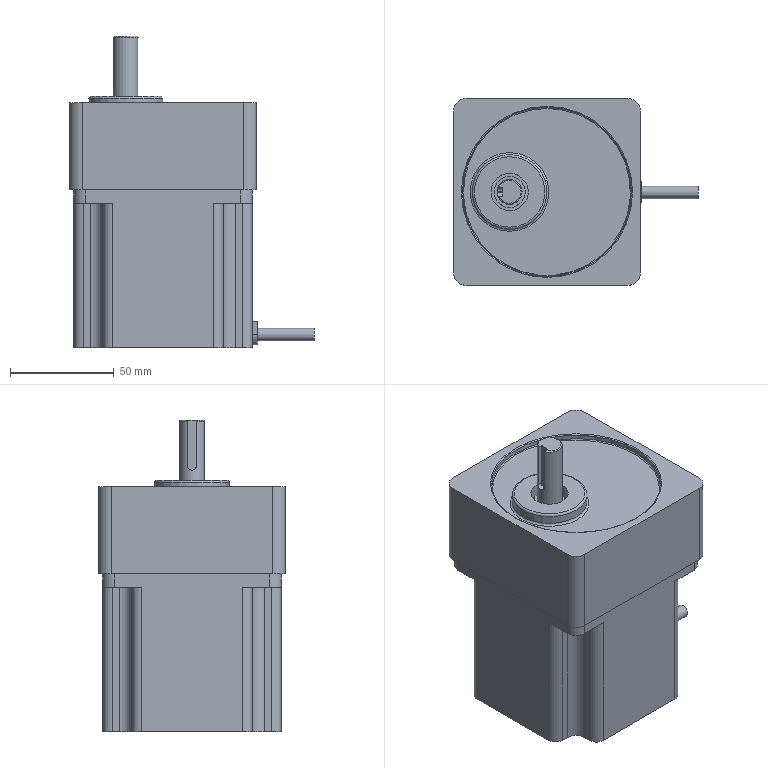Part | NX | features 5003_109_Stepper motor 2 | 1 solid | 81 faces | box 118 x 90 x 150.1 mm | volume 836101 mm3 | plane 38 | cylinder 34 | torus 5 | cone 4 | commonest cylinder face diameters 9.2 x8 12 x5 7 x4 11 x4 11.8 x4 4 x2